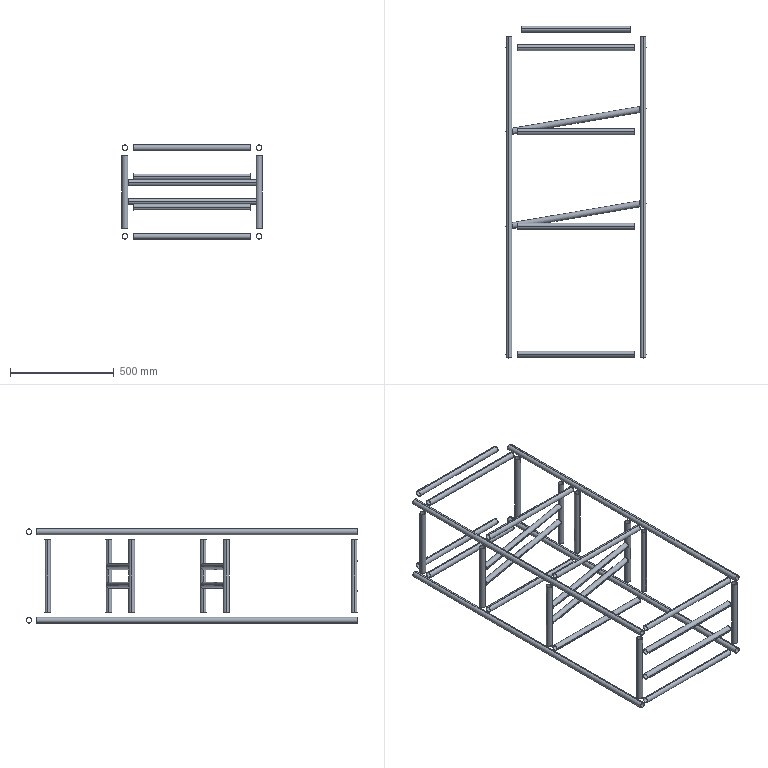Part | STEP file | TUBOS CANASTA_Predeterminado<Como mecanizada> | 30 solids | 180 faces | box 675 x 1600 x 455 mm | volume 1954173 mm3 | cylinder 120 | plane 60 | commonest cylinder face diameters 26.2 x60 28.6 x60